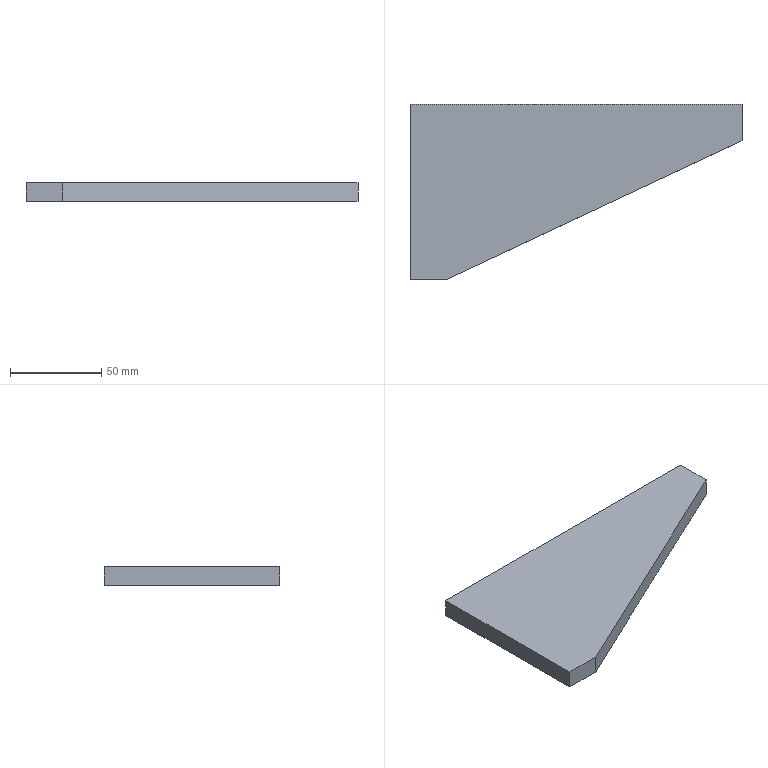Part | STEP file | Reinforcing rib | 1 solid | 7 faces | box 181.9 x 96 x 10 mm | volume 113102 mm3 | plane 7
STEP:
#1=CARTESIAN_POINT('',(0.,0.,-5.));
#2=VERTEX_POINT('',#1);
#3=CARTESIAN_POINT('',(20.,0.,-5.));
#4=VERTEX_POINT('',#3);
#5=CARTESIAN_POINT('',(0.,0.,-5.));
#6=DIRECTION('',(1.,0.,0.));
#7=VECTOR('',#6,1000.);
#8=LINE('',#5,#7);
#9=EDGE_CURVE('',#2,#4,#8,.T.);
#10=ORIENTED_EDGE('',*,*,#9,.T.);
#11=CARTESIAN_POINT('',(20.,0.,5.));
#12=VERTEX_POINT('',#11);
#13=CARTESIAN_POINT('',(20.,0.,5.));
#14=DIRECTION('',(0.,0.,-1.));
#15=VECTOR('',#14,1000.);
#16=LINE('',#13,#15);
#17=EDGE_CURVE('',#12,#4,#16,.T.);
#18=ORIENTED_EDGE('',*,*,#17,.F.);
#19=CARTESIAN_POINT('',(0.,0.,5.));
#20=VERTEX_POINT('',#19);
#21=CARTESIAN_POINT('',(0.,0.,5.));
#22=DIRECTION('',(1.,0.,0.));
#23=VECTOR('',#22,1000.);
#24=LINE('',#21,#23);
#25=EDGE_CURVE('',#20,#12,#24,.T.);
#26=ORIENTED_EDGE('',*,*,#25,.F.);
#27=CARTESIAN_POINT('',(0.,0.,5.));
#28=DIRECTION('',(0.,0.,-1.));
#29=VECTOR('',#28,1000.);
#30=LINE('',#27,#29);
#31=EDGE_CURVE('',#20,#2,#30,.T.);
#32=ORIENTED_EDGE('',*,*,#31,.T.);
#33=EDGE_LOOP('',(#10,#18,#26,#32));
#34=FACE_OUTER_BOUND('',#33,.T.);
#35=CARTESIAN_POINT('',(0.,0.,5.));
#36=DIRECTION('',(0.,1.,0.));
#37=DIRECTION('',(0.,0.,1.));
#38=AXIS2_PLACEMENT_3D('',#35,#36,#37);
#39=PLANE('',#38);
#40=ADVANCED_FACE('',(#34),#39,.F.);
#41=CARTESIAN_POINT('',(181.9,76.,-5.));
#42=VERTEX_POINT('',#41);
#43=CARTESIAN_POINT('',(20.,0.,-5.));
#44=DIRECTION('',(0.9052,0.4249,0.));
#45=VECTOR('',#44,1000.);
#46=LINE('',#43,#45);
#47=EDGE_CURVE('',#4,#42,#46,.T.);
#48=ORIENTED_EDGE('',*,*,#47,.T.);
#49=CARTESIAN_POINT('',(181.9,76.,5.));
#50=VERTEX_POINT('',#49);
#51=CARTESIAN_POINT('',(181.9,76.,5.));
#52=DIRECTION('',(0.,0.,-1.));
#53=VECTOR('',#52,1000.);
#54=LINE('',#51,#53);
#55=EDGE_CURVE('',#50,#42,#54,.T.);
#56=ORIENTED_EDGE('',*,*,#55,.F.);
#57=CARTESIAN_POINT('',(20.,0.,5.));
#58=DIRECTION('',(0.9052,0.4249,0.));
#59=VECTOR('',#58,1000.);
#60=LINE('',#57,#59);
#61=EDGE_CURVE('',#12,#50,#60,.T.);
#62=ORIENTED_EDGE('',*,*,#61,.F.);
#63=ORIENTED_EDGE('',*,*,#17,.T.);
#64=EDGE_LOOP('',(#48,#56,#62,#63));
#65=FACE_OUTER_BOUND('',#64,.T.);
#66=CARTESIAN_POINT('',(20.,0.,5.));
#67=DIRECTION('',(-0.4249,0.9052,0.));
#68=DIRECTION('',(-0.9052,-0.4249,0.));
#69=AXIS2_PLACEMENT_3D('',#66,#67,#68);
#70=PLANE('',#69);
#71=ADVANCED_FACE('',(#65),#70,.F.);
#72=CARTESIAN_POINT('',(181.9,96.,-5.));
#73=VERTEX_POINT('',#72);
#74=CARTESIAN_POINT('',(181.9,96.,-5.));
#75=DIRECTION('',(0.,1.,0.));
#76=VECTOR('',#75,1000.);
#77=LINE('',#74,#76);
#78=EDGE_CURVE('',#42,#73,#77,.T.);
#79=ORIENTED_EDGE('',*,*,#78,.T.);
#80=CARTESIAN_POINT('',(181.9,96.,5.));
#81=VERTEX_POINT('',#80);
#82=CARTESIAN_POINT('',(181.9,96.,5.));
#83=DIRECTION('',(0.,0.,-1.));
#84=VECTOR('',#83,1000.);
#85=LINE('',#82,#84);
#86=EDGE_CURVE('',#81,#73,#85,.T.);
#87=ORIENTED_EDGE('',*,*,#86,.F.);
#88=CARTESIAN_POINT('',(181.9,96.,5.));
#89=DIRECTION('',(0.,1.,0.));
#90=VECTOR('',#89,1000.);
#91=LINE('',#88,#90);
#92=EDGE_CURVE('',#50,#81,#91,.T.);
#93=ORIENTED_EDGE('',*,*,#92,.F.);
#94=ORIENTED_EDGE('',*,*,#55,.T.);
#95=EDGE_LOOP('',(#79,#87,#93,#94));
#96=FACE_OUTER_BOUND('',#95,.T.);
#97=CARTESIAN_POINT('',(181.9,96.,5.));
#98=DIRECTION('',(-1.,0.,0.));
#99=DIRECTION('',(0.,0.,1.));
#100=AXIS2_PLACEMENT_3D('',#97,#98,#99);
#101=PLANE('',#100);
#102=ADVANCED_FACE('',(#96),#101,.F.);
#103=CARTESIAN_POINT('',(0.,96.,-5.));
#104=VERTEX_POINT('',#103);
#105=CARTESIAN_POINT('',(0.,96.,-5.));
#106=DIRECTION('',(-1.,0.,0.));
#107=VECTOR('',#106,1000.);
#108=LINE('',#105,#107);
#109=EDGE_CURVE('',#73,#104,#108,.T.);
#110=ORIENTED_EDGE('',*,*,#109,.T.);
#111=CARTESIAN_POINT('',(0.,96.,5.));
#112=VERTEX_POINT('',#111);
#113=CARTESIAN_POINT('',(0.,96.,5.));
#114=DIRECTION('',(0.,0.,-1.));
#115=VECTOR('',#114,1000.);
#116=LINE('',#113,#115);
#117=EDGE_CURVE('',#112,#104,#116,.T.);
#118=ORIENTED_EDGE('',*,*,#117,.F.);
#119=CARTESIAN_POINT('',(0.,96.,5.));
#120=DIRECTION('',(-1.,0.,0.));
#121=VECTOR('',#120,1000.);
#122=LINE('',#119,#121);
#123=EDGE_CURVE('',#81,#112,#122,.T.);
#124=ORIENTED_EDGE('',*,*,#123,.F.);
#125=ORIENTED_EDGE('',*,*,#86,.T.);
#126=EDGE_LOOP('',(#110,#118,#124,#125));
#127=FACE_OUTER_BOUND('',#126,.T.);
#128=CARTESIAN_POINT('',(0.,96.,5.));
#129=DIRECTION('',(0.,-1.,0.));
#130=DIRECTION('',(0.,0.,-1.));
#131=AXIS2_PLACEMENT_3D('',#128,#129,#130);
#132=PLANE('',#131);
#133=ADVANCED_FACE('',(#127),#132,.F.);
#134=CARTESIAN_POINT('',(0.,0.,-5.));
#135=DIRECTION('',(0.,-1.,0.));
#136=VECTOR('',#135,1000.);
#137=LINE('',#134,#136);
#138=EDGE_CURVE('',#104,#2,#137,.T.);
#139=ORIENTED_EDGE('',*,*,#138,.T.);
#140=ORIENTED_EDGE('',*,*,#31,.F.);
#141=CARTESIAN_POINT('',(0.,0.,5.));
#142=DIRECTION('',(0.,-1.,0.));
#143=VECTOR('',#142,1000.);
#144=LINE('',#141,#143);
#145=EDGE_CURVE('',#112,#20,#144,.T.);
#146=ORIENTED_EDGE('',*,*,#145,.F.);
#147=ORIENTED_EDGE('',*,*,#117,.T.);
#148=EDGE_LOOP('',(#139,#140,#146,#147));
#149=FACE_OUTER_BOUND('',#148,.T.);
#150=CARTESIAN_POINT('',(0.,0.,5.));
#151=DIRECTION('',(1.,0.,0.));
#152=DIRECTION('',(0.,0.,-1.));
#153=AXIS2_PLACEMENT_3D('',#150,#151,#152);
#154=PLANE('',#153);
#155=ADVANCED_FACE('',(#149),#154,.F.);
#156=ORIENTED_EDGE('',*,*,#25,.T.);
#157=ORIENTED_EDGE('',*,*,#61,.T.);
#158=ORIENTED_EDGE('',*,*,#92,.T.);
#159=ORIENTED_EDGE('',*,*,#123,.T.);
#160=ORIENTED_EDGE('',*,*,#145,.T.);
#161=EDGE_LOOP('',(#156,#157,#158,#159,#160));
#162=FACE_OUTER_BOUND('',#161,.T.);
#163=CARTESIAN_POINT('',(0.,0.,5.));
#164=DIRECTION('',(0.,0.,-1.));
#165=DIRECTION('',(-1.,0.,0.));
#166=AXIS2_PLACEMENT_3D('',#163,#164,#165);
#167=PLANE('',#166);
#168=ADVANCED_FACE('',(#162),#167,.F.);
#169=ORIENTED_EDGE('',*,*,#9,.F.);
#170=ORIENTED_EDGE('',*,*,#138,.F.);
#171=ORIENTED_EDGE('',*,*,#109,.F.);
#172=ORIENTED_EDGE('',*,*,#78,.F.);
#173=ORIENTED_EDGE('',*,*,#47,.F.);
#174=EDGE_LOOP('',(#169,#170,#171,#172,#173));
#175=FACE_OUTER_BOUND('',#174,.T.);
#176=CARTESIAN_POINT('',(0.,0.,-5.));
#177=DIRECTION('',(0.,0.,-1.));
#178=DIRECTION('',(-1.,0.,0.));
#179=AXIS2_PLACEMENT_3D('',#176,#177,#178);
#180=PLANE('',#179);
#181=ADVANCED_FACE('',(#175),#180,.T.);
#182=CLOSED_SHELL('',(#40,#71,#102,#133,#155,#168,#181));
#183=MANIFOLD_SOLID_BREP('',#182);
#184=CARTESIAN_POINT('',(0.,0.,0.));
#185=DIRECTION('',(0.,0.,1.));
#186=DIRECTION('',(1.,0.,0.));
#187=AXIS2_PLACEMENT_3D('',#184,#185,#186);
#188=(LENGTH_UNIT()NAMED_UNIT(*)SI_UNIT(.MILLI.,.METRE.));
#189=UNCERTAINTY_MEASURE_WITH_UNIT(LENGTH_MEASURE(0.00001),#188,'','');
#190=(NAMED_UNIT(*)PLANE_ANGLE_UNIT()SI_UNIT($,.RADIAN.));
#191=(NAMED_UNIT(*)SI_UNIT($,.STERADIAN.)SOLID_ANGLE_UNIT());
#192=(GEOMETRIC_REPRESENTATION_CONTEXT(3)GLOBAL_UNCERTAINTY_ASSIGNED_CONTEXT((#189))GLOBAL_UNIT_ASSIGNED_CONTEXT((#188,#190,#191))REPRESENTATION_CONTEXT('',''));
#193=ADVANCED_BREP_SHAPE_REPRESENTATION('',(#183,#187),#192);